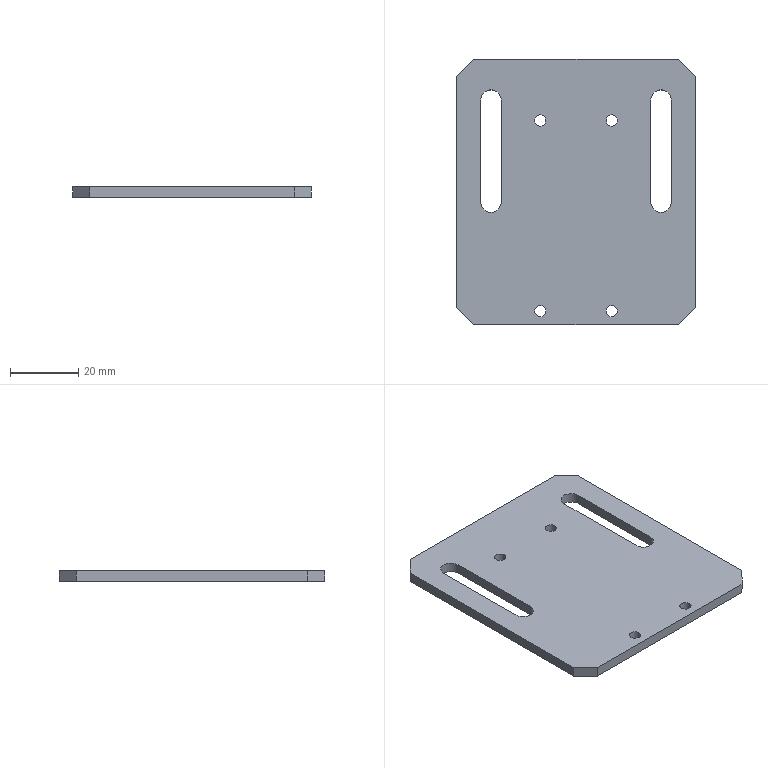Part | SolidWorks | features BaseBody 1 | 1 solid | 26 faces | box 70 x 78 x 3 mm | volume 14878 mm3 | plane 14 | cylinder 12 | commonest cylinder face diameters 3.3 x8 6 x4
STEP:
#1=CARTESIAN_POINT('',(8.85,-35.,-3.));
#2=VERTEX_POINT('',#1);
#3=CARTESIAN_POINT('',(12.15,-35.,-3.));
#4=VERTEX_POINT('',#3);
#5=CARTESIAN_POINT('',(10.5,-35.,-3.));
#6=DIRECTION('',(0.,0.,1.));
#7=DIRECTION('',(1.,0.,0.));
#8=AXIS2_PLACEMENT_3D('',#5,#6,#7);
#9=CIRCLE('',#8,1.65);
#10=EDGE_CURVE('',#2,#4,#9,.T.);
#11=ORIENTED_EDGE('',*,*,#10,.F.);
#12=CARTESIAN_POINT('',(8.85,-35.,0.));
#13=VERTEX_POINT('',#12);
#14=CARTESIAN_POINT('',(8.85,-35.,0.));
#15=DIRECTION('',(0.,0.,1.));
#16=VECTOR('',#15,1000.);
#17=LINE('',#14,#16);
#18=EDGE_CURVE('',#2,#13,#17,.T.);
#19=ORIENTED_EDGE('',*,*,#18,.T.);
#20=CARTESIAN_POINT('',(12.15,-35.,0.));
#21=VERTEX_POINT('',#20);
#22=CARTESIAN_POINT('',(10.5,-35.,0.));
#23=DIRECTION('',(0.,0.,-1.));
#24=DIRECTION('',(1.,0.,0.));
#25=AXIS2_PLACEMENT_3D('',#22,#23,#24);
#26=CIRCLE('',#25,1.65);
#27=EDGE_CURVE('',#21,#13,#26,.T.);
#28=ORIENTED_EDGE('',*,*,#27,.F.);
#29=CARTESIAN_POINT('',(12.15,-35.,0.));
#30=DIRECTION('',(0.,0.,1.));
#31=VECTOR('',#30,1000.);
#32=LINE('',#29,#31);
#33=EDGE_CURVE('',#4,#21,#32,.T.);
#34=ORIENTED_EDGE('',*,*,#33,.F.);
#35=EDGE_LOOP('',(#11,#19,#28,#34));
#36=FACE_OUTER_BOUND('',#35,.T.);
#37=CARTESIAN_POINT('',(10.5,-35.,0.));
#38=DIRECTION('',(0.,0.,1.));
#39=DIRECTION('',(1.,0.,0.));
#40=AXIS2_PLACEMENT_3D('',#37,#38,#39);
#41=CYLINDRICAL_SURFACE('',#40,1.65);
#42=ADVANCED_FACE('',(#36),#41,.F.);
#43=CARTESIAN_POINT('',(-12.15,-35.,-3.));
#44=VERTEX_POINT('',#43);
#45=CARTESIAN_POINT('',(-8.85,-35.,-3.));
#46=VERTEX_POINT('',#45);
#47=CARTESIAN_POINT('',(-10.5,-35.,-3.));
#48=DIRECTION('',(0.,0.,1.));
#49=DIRECTION('',(1.,0.,0.));
#50=AXIS2_PLACEMENT_3D('',#47,#48,#49);
#51=CIRCLE('',#50,1.65);
#52=EDGE_CURVE('',#44,#46,#51,.T.);
#53=ORIENTED_EDGE('',*,*,#52,.F.);
#54=CARTESIAN_POINT('',(-12.15,-35.,0.));
#55=VERTEX_POINT('',#54);
#56=CARTESIAN_POINT('',(-12.15,-35.,0.));
#57=DIRECTION('',(0.,0.,1.));
#58=VECTOR('',#57,1000.);
#59=LINE('',#56,#58);
#60=EDGE_CURVE('',#44,#55,#59,.T.);
#61=ORIENTED_EDGE('',*,*,#60,.T.);
#62=CARTESIAN_POINT('',(-8.85,-35.,0.));
#63=VERTEX_POINT('',#62);
#64=CARTESIAN_POINT('',(-10.5,-35.,0.));
#65=DIRECTION('',(0.,0.,-1.));
#66=DIRECTION('',(1.,0.,0.));
#67=AXIS2_PLACEMENT_3D('',#64,#65,#66);
#68=CIRCLE('',#67,1.65);
#69=EDGE_CURVE('',#63,#55,#68,.T.);
#70=ORIENTED_EDGE('',*,*,#69,.F.);
#71=CARTESIAN_POINT('',(-8.85,-35.,0.));
#72=DIRECTION('',(0.,0.,1.));
#73=VECTOR('',#72,1000.);
#74=LINE('',#71,#73);
#75=EDGE_CURVE('',#46,#63,#74,.T.);
#76=ORIENTED_EDGE('',*,*,#75,.F.);
#77=EDGE_LOOP('',(#53,#61,#70,#76));
#78=FACE_OUTER_BOUND('',#77,.T.);
#79=CARTESIAN_POINT('',(-10.5,-35.,0.));
#80=DIRECTION('',(0.,0.,1.));
#81=DIRECTION('',(1.,0.,0.));
#82=AXIS2_PLACEMENT_3D('',#79,#80,#81);
#83=CYLINDRICAL_SURFACE('',#82,1.65);
#84=ADVANCED_FACE('',(#78),#83,.F.);
#85=CARTESIAN_POINT('',(8.85,21.,-3.));
#86=VERTEX_POINT('',#85);
#87=CARTESIAN_POINT('',(12.15,21.,-3.));
#88=VERTEX_POINT('',#87);
#89=CARTESIAN_POINT('',(10.5,21.,-3.));
#90=DIRECTION('',(0.,0.,1.));
#91=DIRECTION('',(1.,0.,0.));
#92=AXIS2_PLACEMENT_3D('',#89,#90,#91);
#93=CIRCLE('',#92,1.65);
#94=EDGE_CURVE('',#86,#88,#93,.T.);
#95=ORIENTED_EDGE('',*,*,#94,.F.);
#96=CARTESIAN_POINT('',(8.85,21.,0.));
#97=VERTEX_POINT('',#96);
#98=CARTESIAN_POINT('',(8.85,21.,0.));
#99=DIRECTION('',(0.,0.,1.));
#100=VECTOR('',#99,1000.);
#101=LINE('',#98,#100);
#102=EDGE_CURVE('',#86,#97,#101,.T.);
#103=ORIENTED_EDGE('',*,*,#102,.T.);
#104=CARTESIAN_POINT('',(12.15,21.,0.));
#105=VERTEX_POINT('',#104);
#106=CARTESIAN_POINT('',(10.5,21.,0.));
#107=DIRECTION('',(0.,0.,-1.));
#108=DIRECTION('',(1.,0.,0.));
#109=AXIS2_PLACEMENT_3D('',#106,#107,#108);
#110=CIRCLE('',#109,1.65);
#111=EDGE_CURVE('',#105,#97,#110,.T.);
#112=ORIENTED_EDGE('',*,*,#111,.F.);
#113=CARTESIAN_POINT('',(12.15,21.,0.));
#114=DIRECTION('',(0.,0.,1.));
#115=VECTOR('',#114,1000.);
#116=LINE('',#113,#115);
#117=EDGE_CURVE('',#88,#105,#116,.T.);
#118=ORIENTED_EDGE('',*,*,#117,.F.);
#119=EDGE_LOOP('',(#95,#103,#112,#118));
#120=FACE_OUTER_BOUND('',#119,.T.);
#121=CARTESIAN_POINT('',(10.5,21.,0.));
#122=DIRECTION('',(0.,0.,1.));
#123=DIRECTION('',(1.,0.,0.));
#124=AXIS2_PLACEMENT_3D('',#121,#122,#123);
#125=CYLINDRICAL_SURFACE('',#124,1.65);
#126=ADVANCED_FACE('',(#120),#125,.F.);
#127=CARTESIAN_POINT('',(-12.15,21.,-3.));
#128=VERTEX_POINT('',#127);
#129=CARTESIAN_POINT('',(-8.85,21.,-3.));
#130=VERTEX_POINT('',#129);
#131=CARTESIAN_POINT('',(-10.5,21.,-3.));
#132=DIRECTION('',(0.,0.,1.));
#133=DIRECTION('',(1.,0.,0.));
#134=AXIS2_PLACEMENT_3D('',#131,#132,#133);
#135=CIRCLE('',#134,1.65);
#136=EDGE_CURVE('',#128,#130,#135,.T.);
#137=ORIENTED_EDGE('',*,*,#136,.F.);
#138=CARTESIAN_POINT('',(-12.15,21.,0.));
#139=VERTEX_POINT('',#138);
#140=CARTESIAN_POINT('',(-12.15,21.,0.));
#141=DIRECTION('',(0.,0.,1.));
#142=VECTOR('',#141,1000.);
#143=LINE('',#140,#142);
#144=EDGE_CURVE('',#128,#139,#143,.T.);
#145=ORIENTED_EDGE('',*,*,#144,.T.);
#146=CARTESIAN_POINT('',(-8.85,21.,0.));
#147=VERTEX_POINT('',#146);
#148=CARTESIAN_POINT('',(-10.5,21.,0.));
#149=DIRECTION('',(0.,0.,-1.));
#150=DIRECTION('',(1.,0.,0.));
#151=AXIS2_PLACEMENT_3D('',#148,#149,#150);
#152=CIRCLE('',#151,1.65);
#153=EDGE_CURVE('',#147,#139,#152,.T.);
#154=ORIENTED_EDGE('',*,*,#153,.F.);
#155=CARTESIAN_POINT('',(-8.85,21.,0.));
#156=DIRECTION('',(0.,0.,1.));
#157=VECTOR('',#156,1000.);
#158=LINE('',#155,#157);
#159=EDGE_CURVE('',#130,#147,#158,.T.);
#160=ORIENTED_EDGE('',*,*,#159,.F.);
#161=EDGE_LOOP('',(#137,#145,#154,#160));
#162=FACE_OUTER_BOUND('',#161,.T.);
#163=CARTESIAN_POINT('',(-10.5,21.,0.));
#164=DIRECTION('',(0.,0.,1.));
#165=DIRECTION('',(1.,0.,0.));
#166=AXIS2_PLACEMENT_3D('',#163,#164,#165);
#167=CYLINDRICAL_SURFACE('',#166,1.65);
#168=ADVANCED_FACE('',(#162),#167,.F.);
#169=CARTESIAN_POINT('',(30.,39.,0.));
#170=VERTEX_POINT('',#169);
#171=CARTESIAN_POINT('',(-30.,39.,0.));
#172=VERTEX_POINT('',#171);
#173=CARTESIAN_POINT('',(0.,39.,0.));
#174=DIRECTION('',(-1.,0.,0.));
#175=VECTOR('',#174,1000.);
#176=LINE('',#173,#175);
#177=EDGE_CURVE('',#170,#172,#176,.T.);
#178=ORIENTED_EDGE('',*,*,#177,.T.);
#179=CARTESIAN_POINT('',(-35.,34.,0.));
#180=VERTEX_POINT('',#179);
#181=CARTESIAN_POINT('',(-30.,39.,0.));
#182=DIRECTION('',(-0.7071,-0.7071,0.));
#183=VECTOR('',#182,1000.);
#184=LINE('',#181,#183);
#185=EDGE_CURVE('',#172,#180,#184,.T.);
#186=ORIENTED_EDGE('',*,*,#185,.T.);
#187=CARTESIAN_POINT('',(-35.,-34.,0.));
#188=VERTEX_POINT('',#187);
#189=CARTESIAN_POINT('',(-35.,0.,0.));
#190=DIRECTION('',(0.,-1.,0.));
#191=VECTOR('',#190,1000.);
#192=LINE('',#189,#191);
#193=EDGE_CURVE('',#180,#188,#192,.T.);
#194=ORIENTED_EDGE('',*,*,#193,.T.);
#195=CARTESIAN_POINT('',(-30.,-39.,0.));
#196=VERTEX_POINT('',#195);
#197=CARTESIAN_POINT('',(-35.,-34.,0.));
#198=DIRECTION('',(0.7071,-0.7071,0.));
#199=VECTOR('',#198,1000.);
#200=LINE('',#197,#199);
#201=EDGE_CURVE('',#188,#196,#200,.T.);
#202=ORIENTED_EDGE('',*,*,#201,.T.);
#203=CARTESIAN_POINT('',(30.,-39.,0.));
#204=VERTEX_POINT('',#203);
#205=CARTESIAN_POINT('',(0.,-39.,0.));
#206=DIRECTION('',(1.,0.,0.));
#207=VECTOR('',#206,1000.);
#208=LINE('',#205,#207);
#209=EDGE_CURVE('',#196,#204,#208,.T.);
#210=ORIENTED_EDGE('',*,*,#209,.T.);
#211=CARTESIAN_POINT('',(35.,-34.,0.));
#212=VERTEX_POINT('',#211);
#213=CARTESIAN_POINT('',(30.,-39.,0.));
#214=DIRECTION('',(0.7071,0.7071,0.));
#215=VECTOR('',#214,1000.);
#216=LINE('',#213,#215);
#217=EDGE_CURVE('',#204,#212,#216,.T.);
#218=ORIENTED_EDGE('',*,*,#217,.T.);
#219=CARTESIAN_POINT('',(35.,34.,0.));
#220=VERTEX_POINT('',#219);
#221=CARTESIAN_POINT('',(35.,0.,0.));
#222=DIRECTION('',(0.,1.,0.));
#223=VECTOR('',#222,1000.);
#224=LINE('',#221,#223);
#225=EDGE_CURVE('',#212,#220,#224,.T.);
#226=ORIENTED_EDGE('',*,*,#225,.T.);
#227=CARTESIAN_POINT('',(35.,34.,0.));
#228=DIRECTION('',(-0.7071,0.7071,0.));
#229=VECTOR('',#228,1000.);
#230=LINE('',#227,#229);
#231=EDGE_CURVE('',#220,#170,#230,.T.);
#232=ORIENTED_EDGE('',*,*,#231,.T.);
#233=EDGE_LOOP('',(#178,#186,#194,#202,#210,#218,#226,#232));
#234=FACE_OUTER_BOUND('',#233,.T.);
#235=ORIENTED_EDGE('',*,*,#27,.T.);
#236=CARTESIAN_POINT('',(10.5,-35.,0.));
#237=DIRECTION('',(0.,0.,-1.));
#238=DIRECTION('',(1.,0.,0.));
#239=AXIS2_PLACEMENT_3D('',#236,#237,#238);
#240=CIRCLE('',#239,1.65);
#241=EDGE_CURVE('',#13,#21,#240,.T.);
#242=ORIENTED_EDGE('',*,*,#241,.T.);
#243=EDGE_LOOP('',(#235,#242));
#244=FACE_BOUND('',#243,.T.);
#245=ORIENTED_EDGE('',*,*,#69,.T.);
#246=CARTESIAN_POINT('',(-10.5,-35.,0.));
#247=DIRECTION('',(0.,0.,-1.));
#248=DIRECTION('',(1.,0.,0.));
#249=AXIS2_PLACEMENT_3D('',#246,#247,#248);
#250=CIRCLE('',#249,1.65);
#251=EDGE_CURVE('',#55,#63,#250,.T.);
#252=ORIENTED_EDGE('',*,*,#251,.T.);
#253=EDGE_LOOP('',(#245,#252));
#254=FACE_BOUND('',#253,.T.);
#255=ORIENTED_EDGE('',*,*,#111,.T.);
#256=CARTESIAN_POINT('',(10.5,21.,0.));
#257=DIRECTION('',(0.,0.,-1.));
#258=DIRECTION('',(1.,0.,0.));
#259=AXIS2_PLACEMENT_3D('',#256,#257,#258);
#260=CIRCLE('',#259,1.65);
#261=EDGE_CURVE('',#97,#105,#260,.T.);
#262=ORIENTED_EDGE('',*,*,#261,.T.);
#263=EDGE_LOOP('',(#255,#262));
#264=FACE_BOUND('',#263,.T.);
#265=ORIENTED_EDGE('',*,*,#153,.T.);
#266=CARTESIAN_POINT('',(-10.5,21.,0.));
#267=DIRECTION('',(0.,0.,-1.));
#268=DIRECTION('',(1.,0.,0.));
#269=AXIS2_PLACEMENT_3D('',#266,#267,#268);
#270=CIRCLE('',#269,1.65);
#271=EDGE_CURVE('',#139,#147,#270,.T.);
#272=ORIENTED_EDGE('',*,*,#271,.T.);
#273=EDGE_LOOP('',(#265,#272));
#274=FACE_BOUND('',#273,.T.);
#275=CARTESIAN_POINT('',(-22.,-3.,0.));
#276=VERTEX_POINT('',#275);
#277=CARTESIAN_POINT('',(-28.,-3.,0.));
#278=VERTEX_POINT('',#277);
#279=CARTESIAN_POINT('',(-25.,-3.,0.));
#280=DIRECTION('',(0.,0.,-1.));
#281=DIRECTION('',(1.,0.,0.));
#282=AXIS2_PLACEMENT_3D('',#279,#280,#281);
#283=CIRCLE('',#282,3.);
#284=EDGE_CURVE('',#276,#278,#283,.T.);
#285=ORIENTED_EDGE('',*,*,#284,.T.);
#286=CARTESIAN_POINT('',(-28.,27.,0.));
#287=VERTEX_POINT('',#286);
#288=CARTESIAN_POINT('',(-28.,0.,0.));
#289=DIRECTION('',(0.,1.,0.));
#290=VECTOR('',#289,1000.);
#291=LINE('',#288,#290);
#292=EDGE_CURVE('',#278,#287,#291,.T.);
#293=ORIENTED_EDGE('',*,*,#292,.T.);
#294=CARTESIAN_POINT('',(-22.,27.,0.));
#295=VERTEX_POINT('',#294);
#296=CARTESIAN_POINT('',(-25.,27.,0.));
#297=DIRECTION('',(0.,0.,-1.));
#298=DIRECTION('',(1.,0.,0.));
#299=AXIS2_PLACEMENT_3D('',#296,#297,#298);
#300=CIRCLE('',#299,3.);
#301=EDGE_CURVE('',#287,#295,#300,.T.);
#302=ORIENTED_EDGE('',*,*,#301,.T.);
#303=CARTESIAN_POINT('',(-22.,0.,0.));
#304=DIRECTION('',(0.,-1.,0.));
#305=VECTOR('',#304,1000.);
#306=LINE('',#303,#305);
#307=EDGE_CURVE('',#295,#276,#306,.T.);
#308=ORIENTED_EDGE('',*,*,#307,.T.);
#309=EDGE_LOOP('',(#285,#293,#302,#308));
#310=FACE_BOUND('',#309,.T.);
#311=CARTESIAN_POINT('',(28.,-3.,0.));
#312=VERTEX_POINT('',#311);
#313=CARTESIAN_POINT('',(22.,-3.,0.));
#314=VERTEX_POINT('',#313);
#315=CARTESIAN_POINT('',(25.,-3.,0.));
#316=DIRECTION('',(0.,0.,-1.));
#317=DIRECTION('',(1.,0.,0.));
#318=AXIS2_PLACEMENT_3D('',#315,#316,#317);
#319=CIRCLE('',#318,3.);
#320=EDGE_CURVE('',#312,#314,#319,.T.);
#321=ORIENTED_EDGE('',*,*,#320,.T.);
#322=CARTESIAN_POINT('',(22.,27.,0.));
#323=VERTEX_POINT('',#322);
#324=CARTESIAN_POINT('',(22.,0.,0.));
#325=DIRECTION('',(0.,1.,0.));
#326=VECTOR('',#325,1000.);
#327=LINE('',#324,#326);
#328=EDGE_CURVE('',#314,#323,#327,.T.);
#329=ORIENTED_EDGE('',*,*,#328,.T.);
#330=CARTESIAN_POINT('',(28.,27.,0.));
#331=VERTEX_POINT('',#330);
#332=CARTESIAN_POINT('',(25.,27.,0.));
#333=DIRECTION('',(0.,0.,-1.));
#334=DIRECTION('',(1.,0.,0.));
#335=AXIS2_PLACEMENT_3D('',#332,#333,#334);
#336=CIRCLE('',#335,3.);
#337=EDGE_CURVE('',#323,#331,#336,.T.);
#338=ORIENTED_EDGE('',*,*,#337,.T.);
#339=CARTESIAN_POINT('',(28.,0.,0.));
#340=DIRECTION('',(0.,-1.,0.));
#341=VECTOR('',#340,1000.);
#342=LINE('',#339,#341);
#343=EDGE_CURVE('',#331,#312,#342,.T.);
#344=ORIENTED_EDGE('',*,*,#343,.T.);
#345=EDGE_LOOP('',(#321,#329,#338,#344));
#346=FACE_BOUND('',#345,.T.);
#347=CARTESIAN_POINT('',(0.,0.,0.));
#348=DIRECTION('',(0.,0.,1.));
#349=DIRECTION('',(1.,0.,0.));
#350=AXIS2_PLACEMENT_3D('',#347,#348,#349);
#351=PLANE('',#350);
#352=ADVANCED_FACE('',(#234,#244,#254,#264,#274,#310,#346),#351,.T.);
#353=CARTESIAN_POINT('',(-35.,34.,-3.));
#354=VERTEX_POINT('',#353);
#355=CARTESIAN_POINT('',(-35.,34.,-3.));
#356=DIRECTION('',(0.,0.,-1.));
#357=VECTOR('',#356,1000.);
#358=LINE('',#355,#357);
#359=EDGE_CURVE('',#180,#354,#358,.T.);
#360=ORIENTED_EDGE('',*,*,#359,.F.);
#361=ORIENTED_EDGE('',*,*,#185,.F.);
#362=CARTESIAN_POINT('',(-30.,39.,-3.));
#363=VERTEX_POINT('',#362);
#364=CARTESIAN_POINT('',(-30.,39.,-3.));
#365=DIRECTION('',(0.,0.,1.));
#366=VECTOR('',#365,1000.);
#367=LINE('',#364,#366);
#368=EDGE_CURVE('',#363,#172,#367,.T.);
#369=ORIENTED_EDGE('',*,*,#368,.F.);
#370=CARTESIAN_POINT('',(-30.,39.,-3.));
#371=DIRECTION('',(0.7071,0.7071,0.));
#372=VECTOR('',#371,1000.);
#373=LINE('',#370,#372);
#374=EDGE_CURVE('',#354,#363,#373,.T.);
#375=ORIENTED_EDGE('',*,*,#374,.F.);
#376=EDGE_LOOP('',(#360,#361,#369,#375));
#377=FACE_OUTER_BOUND('',#376,.T.);
#378=CARTESIAN_POINT('',(-30.,39.,-3.));
#379=DIRECTION('',(0.7071,-0.7071,0.));
#380=DIRECTION('',(0.7071,0.7071,0.));
#381=AXIS2_PLACEMENT_3D('',#378,#379,#380);
#382=PLANE('',#381);
#383=ADVANCED_FACE('',(#377),#382,.F.);
#384=CARTESIAN_POINT('',(30.,39.,-3.));
#385=VERTEX_POINT('',#384);
#386=CARTESIAN_POINT('',(-35.,39.,-3.));
#387=DIRECTION('',(-1.,0.,0.));
#388=VECTOR('',#387,1000.);
#389=LINE('',#386,#388);
#390=EDGE_CURVE('',#385,#363,#389,.T.);
#391=ORIENTED_EDGE('',*,*,#390,.T.);
#392=ORIENTED_EDGE('',*,*,#368,.T.);
#393=ORIENTED_EDGE('',*,*,#177,.F.);
#394=CARTESIAN_POINT('',(30.,39.,-3.));
#395=DIRECTION('',(0.,0.,-1.));
#396=VECTOR('',#395,1000.);
#397=LINE('',#394,#396);
#398=EDGE_CURVE('',#170,#385,#397,.T.);
#399=ORIENTED_EDGE('',*,*,#398,.T.);
#400=EDGE_LOOP('',(#391,#392,#393,#399));
#401=FACE_OUTER_BOUND('',#400,.T.);
#402=CARTESIAN_POINT('',(-35.,39.,-3.));
#403=DIRECTION('',(0.,1.,0.));
#404=DIRECTION('',(0.,0.,1.));
#405=AXIS2_PLACEMENT_3D('',#402,#403,#404);
#406=PLANE('',#405);
#407=ADVANCED_FACE('',(#401),#406,.T.);
#408=ORIENTED_EDGE('',*,*,#398,.F.);
#409=ORIENTED_EDGE('',*,*,#231,.F.);
#410=CARTESIAN_POINT('',(35.,34.,-3.));
#411=VERTEX_POINT('',#410);
#412=CARTESIAN_POINT('',(35.,34.,-3.));
#413=DIRECTION('',(0.,0.,1.));
#414=VECTOR('',#413,1000.);
#415=LINE('',#412,#414);
#416=EDGE_CURVE('',#411,#220,#415,.T.);
#417=ORIENTED_EDGE('',*,*,#416,.F.);
#418=CARTESIAN_POINT('',(35.,34.,-3.));
#419=DIRECTION('',(0.7071,-0.7071,0.));
#420=VECTOR('',#419,1000.);
#421=LINE('',#418,#420);
#422=EDGE_CURVE('',#385,#411,#421,.T.);
#423=ORIENTED_EDGE('',*,*,#422,.F.);
#424=EDGE_LOOP('',(#408,#409,#417,#423));
#425=FACE_OUTER_BOUND('',#424,.T.);
#426=CARTESIAN_POINT('',(35.,34.,-3.));
#427=DIRECTION('',(-0.7071,-0.7071,0.));
#428=DIRECTION('',(0.7071,-0.7071,0.));
#429=AXIS2_PLACEMENT_3D('',#426,#427,#428);
#430=PLANE('',#429);
#431=ADVANCED_FACE('',(#425),#430,.F.);
#432=CARTESIAN_POINT('',(35.,-34.,-3.));
#433=VERTEX_POINT('',#432);
#434=CARTESIAN_POINT('',(35.,39.,-3.));
#435=DIRECTION('',(0.,1.,0.));
#436=VECTOR('',#435,1000.);
#437=LINE('',#434,#436);
#438=EDGE_CURVE('',#433,#411,#437,.T.);
#439=ORIENTED_EDGE('',*,*,#438,.T.);
#440=ORIENTED_EDGE('',*,*,#416,.T.);
#441=ORIENTED_EDGE('',*,*,#225,.F.);
#442=CARTESIAN_POINT('',(35.,-34.,-3.));
#443=DIRECTION('',(0.,0.,-1.));
#444=VECTOR('',#443,1000.);
#445=LINE('',#442,#444);
#446=EDGE_CURVE('',#212,#433,#445,.T.);
#447=ORIENTED_EDGE('',*,*,#446,.T.);
#448=EDGE_LOOP('',(#439,#440,#441,#447));
#449=FACE_OUTER_BOUND('',#448,.T.);
#450=CARTESIAN_POINT('',(35.,39.,-3.));
#451=DIRECTION('',(1.,0.,0.));
#452=DIRECTION('',(0.,1.,0.));
#453=AXIS2_PLACEMENT_3D('',#450,#451,#452);
#454=PLANE('',#453);
#455=ADVANCED_FACE('',(#449),#454,.T.);
#456=ORIENTED_EDGE('',*,*,#446,.F.);
#457=ORIENTED_EDGE('',*,*,#217,.F.);
#458=CARTESIAN_POINT('',(30.,-39.,-3.));
#459=VERTEX_POINT('',#458);
#460=CARTESIAN_POINT('',(30.,-39.,-3.));
#461=DIRECTION('',(0.,0.,1.));
#462=VECTOR('',#461,1000.);
#463=LINE('',#460,#462);
#464=EDGE_CURVE('',#459,#204,#463,.T.);
#465=ORIENTED_EDGE('',*,*,#464,.F.);
#466=CARTESIAN_POINT('',(30.,-39.,-3.));
#467=DIRECTION('',(-0.7071,-0.7071,0.));
#468=VECTOR('',#467,1000.);
#469=LINE('',#466,#468);
#470=EDGE_CURVE('',#433,#459,#469,.T.);
#471=ORIENTED_EDGE('',*,*,#470,.F.);
#472=EDGE_LOOP('',(#456,#457,#465,#471));
#473=FACE_OUTER_BOUND('',#472,.T.);
#474=CARTESIAN_POINT('',(30.,-39.,-3.));
#475=DIRECTION('',(-0.7071,0.7071,0.));
#476=DIRECTION('',(-0.7071,-0.7071,0.));
#477=AXIS2_PLACEMENT_3D('',#474,#475,#476);
#478=PLANE('',#477);
#479=ADVANCED_FACE('',(#473),#478,.F.);
#480=CARTESIAN_POINT('',(-30.,-39.,-3.));
#481=VERTEX_POINT('',#480);
#482=CARTESIAN_POINT('',(-35.,-39.,-3.));
#483=DIRECTION('',(1.,0.,0.));
#484=VECTOR('',#483,1000.);
#485=LINE('',#482,#484);
#486=EDGE_CURVE('',#481,#459,#485,.T.);
#487=ORIENTED_EDGE('',*,*,#486,.T.);
#488=ORIENTED_EDGE('',*,*,#464,.T.);
#489=ORIENTED_EDGE('',*,*,#209,.F.);
#490=CARTESIAN_POINT('',(-30.,-39.,-3.));
#491=DIRECTION('',(0.,0.,-1.));
#492=VECTOR('',#491,1000.);
#493=LINE('',#490,#492);
#494=EDGE_CURVE('',#196,#481,#493,.T.);
#495=ORIENTED_EDGE('',*,*,#494,.T.);
#496=EDGE_LOOP('',(#487,#488,#489,#495));
#497=FACE_OUTER_BOUND('',#496,.T.);
#498=CARTESIAN_POINT('',(-35.,-39.,-3.));
#499=DIRECTION('',(0.,-1.,0.));
#500=DIRECTION('',(0.,0.,-1.));
#501=AXIS2_PLACEMENT_3D('',#498,#499,#500);
#502=PLANE('',#501);
#503=ADVANCED_FACE('',(#497),#502,.T.);
#504=ORIENTED_EDGE('',*,*,#494,.F.);
#505=ORIENTED_EDGE('',*,*,#201,.F.);
#506=CARTESIAN_POINT('',(-35.,-34.,-3.));
#507=VERTEX_POINT('',#506);
#508=CARTESIAN_POINT('',(-35.,-34.,-3.));
#509=DIRECTION('',(0.,0.,1.));
#510=VECTOR('',#509,1000.);
#511=LINE('',#508,#510);
#512=EDGE_CURVE('',#507,#188,#511,.T.);
#513=ORIENTED_EDGE('',*,*,#512,.F.);
#514=CARTESIAN_POINT('',(-35.,-34.,-3.));
#515=DIRECTION('',(-0.7071,0.7071,0.));
#516=VECTOR('',#515,1000.);
#517=LINE('',#514,#516);
#518=EDGE_CURVE('',#481,#507,#517,.T.);
#519=ORIENTED_EDGE('',*,*,#518,.F.);
#520=EDGE_LOOP('',(#504,#505,#513,#519));
#521=FACE_OUTER_BOUND('',#520,.T.);
#522=CARTESIAN_POINT('',(-35.,-34.,-3.));
#523=DIRECTION('',(0.7071,0.7071,0.));
#524=DIRECTION('',(-0.7071,0.7071,0.));
#525=AXIS2_PLACEMENT_3D('',#522,#523,#524);
#526=PLANE('',#525);
#527=ADVANCED_FACE('',(#521),#526,.F.);
#528=ORIENTED_EDGE('',*,*,#193,.F.);
#529=ORIENTED_EDGE('',*,*,#359,.T.);
#530=CARTESIAN_POINT('',(-35.,39.,-3.));
#531=DIRECTION('',(0.,-1.,0.));
#532=VECTOR('',#531,1000.);
#533=LINE('',#530,#532);
#534=EDGE_CURVE('',#354,#507,#533,.T.);
#535=ORIENTED_EDGE('',*,*,#534,.T.);
#536=ORIENTED_EDGE('',*,*,#512,.T.);
#537=EDGE_LOOP('',(#528,#529,#535,#536));
#538=FACE_OUTER_BOUND('',#537,.T.);
#539=CARTESIAN_POINT('',(-35.,39.,-3.));
#540=DIRECTION('',(-1.,0.,0.));
#541=DIRECTION('',(0.,-1.,0.));
#542=AXIS2_PLACEMENT_3D('',#539,#540,#541);
#543=PLANE('',#542);
#544=ADVANCED_FACE('',(#538),#543,.T.);
#545=ORIENTED_EDGE('',*,*,#18,.F.);
#546=CARTESIAN_POINT('',(10.5,-35.,-3.));
#547=DIRECTION('',(0.,0.,1.));
#548=DIRECTION('',(1.,0.,0.));
#549=AXIS2_PLACEMENT_3D('',#546,#547,#548);
#550=CIRCLE('',#549,1.65);
#551=EDGE_CURVE('',#4,#2,#550,.T.);
#552=ORIENTED_EDGE('',*,*,#551,.F.);
#553=ORIENTED_EDGE('',*,*,#33,.T.);
#554=ORIENTED_EDGE('',*,*,#241,.F.);
#555=EDGE_LOOP('',(#545,#552,#553,#554));
#556=FACE_OUTER_BOUND('',#555,.T.);
#557=CARTESIAN_POINT('',(10.5,-35.,0.));
#558=DIRECTION('',(0.,0.,1.));
#559=DIRECTION('',(1.,0.,0.));
#560=AXIS2_PLACEMENT_3D('',#557,#558,#559);
#561=CYLINDRICAL_SURFACE('',#560,1.65);
#562=ADVANCED_FACE('',(#556),#561,.F.);
#563=ORIENTED_EDGE('',*,*,#60,.F.);
#564=CARTESIAN_POINT('',(-10.5,-35.,-3.));
#565=DIRECTION('',(0.,0.,1.));
#566=DIRECTION('',(1.,0.,0.));
#567=AXIS2_PLACEMENT_3D('',#564,#565,#566);
#568=CIRCLE('',#567,1.65);
#569=EDGE_CURVE('',#46,#44,#568,.T.);
#570=ORIENTED_EDGE('',*,*,#569,.F.);
#571=ORIENTED_EDGE('',*,*,#75,.T.);
#572=ORIENTED_EDGE('',*,*,#251,.F.);
#573=EDGE_LOOP('',(#563,#570,#571,#572));
#574=FACE_OUTER_BOUND('',#573,.T.);
#575=CARTESIAN_POINT('',(-10.5,-35.,0.));
#576=DIRECTION('',(0.,0.,1.));
#577=DIRECTION('',(1.,0.,0.));
#578=AXIS2_PLACEMENT_3D('',#575,#576,#577);
#579=CYLINDRICAL_SURFACE('',#578,1.65);
#580=ADVANCED_FACE('',(#574),#579,.F.);
#581=ORIENTED_EDGE('',*,*,#102,.F.);
#582=CARTESIAN_POINT('',(10.5,21.,-3.));
#583=DIRECTION('',(0.,0.,1.));
#584=DIRECTION('',(1.,0.,0.));
#585=AXIS2_PLACEMENT_3D('',#582,#583,#584);
#586=CIRCLE('',#585,1.65);
#587=EDGE_CURVE('',#88,#86,#586,.T.);
#588=ORIENTED_EDGE('',*,*,#587,.F.);
#589=ORIENTED_EDGE('',*,*,#117,.T.);
#590=ORIENTED_EDGE('',*,*,#261,.F.);
#591=EDGE_LOOP('',(#581,#588,#589,#590));
#592=FACE_OUTER_BOUND('',#591,.T.);
#593=CARTESIAN_POINT('',(10.5,21.,0.));
#594=DIRECTION('',(0.,0.,1.));
#595=DIRECTION('',(1.,0.,0.));
#596=AXIS2_PLACEMENT_3D('',#593,#594,#595);
#597=CYLINDRICAL_SURFACE('',#596,1.65);
#598=ADVANCED_FACE('',(#592),#597,.F.);
#599=ORIENTED_EDGE('',*,*,#144,.F.);
#600=CARTESIAN_POINT('',(-10.5,21.,-3.));
#601=DIRECTION('',(0.,0.,1.));
#602=DIRECTION('',(1.,0.,0.));
#603=AXIS2_PLACEMENT_3D('',#600,#601,#602);
#604=CIRCLE('',#603,1.65);
#605=EDGE_CURVE('',#130,#128,#604,.T.);
#606=ORIENTED_EDGE('',*,*,#605,.F.);
#607=ORIENTED_EDGE('',*,*,#159,.T.);
#608=ORIENTED_EDGE('',*,*,#271,.F.);
#609=EDGE_LOOP('',(#599,#606,#607,#608));
#610=FACE_OUTER_BOUND('',#609,.T.);
#611=CARTESIAN_POINT('',(-10.5,21.,0.));
#612=DIRECTION('',(0.,0.,1.));
#613=DIRECTION('',(1.,0.,0.));
#614=AXIS2_PLACEMENT_3D('',#611,#612,#613);
#615=CYLINDRICAL_SURFACE('',#614,1.65);
#616=ADVANCED_FACE('',(#610),#615,.F.);
#617=CARTESIAN_POINT('',(-28.,-3.,-3.));
#618=VERTEX_POINT('',#617);
#619=CARTESIAN_POINT('',(-28.,-3.,-3.));
#620=DIRECTION('',(0.,0.,1.));
#621=VECTOR('',#620,1000.);
#622=LINE('',#619,#621);
#623=EDGE_CURVE('',#618,#278,#622,.T.);
#624=ORIENTED_EDGE('',*,*,#623,.F.);
#625=CARTESIAN_POINT('',(-28.,27.,-3.));
#626=VERTEX_POINT('',#625);
#627=CARTESIAN_POINT('',(-28.,27.,-3.));
#628=DIRECTION('',(0.,-1.,0.));
#629=VECTOR('',#628,1000.);
#630=LINE('',#627,#629);
#631=EDGE_CURVE('',#626,#618,#630,.T.);
#632=ORIENTED_EDGE('',*,*,#631,.F.);
#633=CARTESIAN_POINT('',(-28.,27.,-3.));
#634=DIRECTION('',(0.,0.,-1.));
#635=VECTOR('',#634,1000.);
#636=LINE('',#633,#635);
#637=EDGE_CURVE('',#287,#626,#636,.T.);
#638=ORIENTED_EDGE('',*,*,#637,.F.);
#639=ORIENTED_EDGE('',*,*,#292,.F.);
#640=EDGE_LOOP('',(#624,#632,#638,#639));
#641=FACE_OUTER_BOUND('',#640,.T.);
#642=CARTESIAN_POINT('',(-28.,27.,-3.));
#643=DIRECTION('',(-1.,0.,0.));
#644=DIRECTION('',(0.,-1.,0.));
#645=AXIS2_PLACEMENT_3D('',#642,#643,#644);
#646=PLANE('',#645);
#647=ADVANCED_FACE('',(#641),#646,.F.);
#648=CARTESIAN_POINT('',(-22.,-3.,-3.));
#649=VERTEX_POINT('',#648);
#650=CARTESIAN_POINT('',(-22.,-3.,-3.));
#651=DIRECTION('',(0.,0.,1.));
#652=VECTOR('',#651,1000.);
#653=LINE('',#650,#652);
#654=EDGE_CURVE('',#649,#276,#653,.T.);
#655=ORIENTED_EDGE('',*,*,#654,.F.);
#656=CARTESIAN_POINT('',(-25.,-3.,-3.));
#657=DIRECTION('',(0.,0.,1.));
#658=DIRECTION('',(1.,0.,0.));
#659=AXIS2_PLACEMENT_3D('',#656,#657,#658);
#660=CIRCLE('',#659,3.);
#661=EDGE_CURVE('',#618,#649,#660,.T.);
#662=ORIENTED_EDGE('',*,*,#661,.F.);
#663=ORIENTED_EDGE('',*,*,#623,.T.);
#664=ORIENTED_EDGE('',*,*,#284,.F.);
#665=EDGE_LOOP('',(#655,#662,#663,#664));
#666=FACE_OUTER_BOUND('',#665,.T.);
#667=CARTESIAN_POINT('',(-25.,-3.,-3.));
#668=DIRECTION('',(0.,0.,1.));
#669=DIRECTION('',(1.,0.,0.));
#670=AXIS2_PLACEMENT_3D('',#667,#668,#669);
#671=CYLINDRICAL_SURFACE('',#670,3.);
#672=ADVANCED_FACE('',(#666),#671,.F.);
#673=CARTESIAN_POINT('',(-22.,27.,-3.));
#674=VERTEX_POINT('',#673);
#675=CARTESIAN_POINT('',(-22.,27.,-3.));
#676=DIRECTION('',(0.,0.,1.));
#677=VECTOR('',#676,1000.);
#678=LINE('',#675,#677);
#679=EDGE_CURVE('',#674,#295,#678,.T.);
#680=ORIENTED_EDGE('',*,*,#679,.F.);
#681=CARTESIAN_POINT('',(-22.,27.,-3.));
#682=DIRECTION('',(0.,1.,0.));
#683=VECTOR('',#682,1000.);
#684=LINE('',#681,#683);
#685=EDGE_CURVE('',#649,#674,#684,.T.);
#686=ORIENTED_EDGE('',*,*,#685,.F.);
#687=ORIENTED_EDGE('',*,*,#654,.T.);
#688=ORIENTED_EDGE('',*,*,#307,.F.);
#689=EDGE_LOOP('',(#680,#686,#687,#688));
#690=FACE_OUTER_BOUND('',#689,.T.);
#691=CARTESIAN_POINT('',(-22.,27.,-3.));
#692=DIRECTION('',(1.,0.,0.));
#693=DIRECTION('',(0.,1.,0.));
#694=AXIS2_PLACEMENT_3D('',#691,#692,#693);
#695=PLANE('',#694);
#696=ADVANCED_FACE('',(#690),#695,.F.);
#697=ORIENTED_EDGE('',*,*,#637,.T.);
#698=CARTESIAN_POINT('',(-25.,27.,-3.));
#699=DIRECTION('',(0.,0.,1.));
#700=DIRECTION('',(1.,0.,0.));
#701=AXIS2_PLACEMENT_3D('',#698,#699,#700);
#702=CIRCLE('',#701,3.);
#703=EDGE_CURVE('',#674,#626,#702,.T.);
#704=ORIENTED_EDGE('',*,*,#703,.F.);
#705=ORIENTED_EDGE('',*,*,#679,.T.);
#706=ORIENTED_EDGE('',*,*,#301,.F.);
#707=EDGE_LOOP('',(#697,#704,#705,#706));
#708=FACE_OUTER_BOUND('',#707,.T.);
#709=CARTESIAN_POINT('',(-25.,27.,-3.));
#710=DIRECTION('',(0.,0.,1.));
#711=DIRECTION('',(1.,0.,0.));
#712=AXIS2_PLACEMENT_3D('',#709,#710,#711);
#713=CYLINDRICAL_SURFACE('',#712,3.);
#714=ADVANCED_FACE('',(#708),#713,.F.);
#715=CARTESIAN_POINT('',(22.,-3.,-3.));
#716=VERTEX_POINT('',#715);
#717=CARTESIAN_POINT('',(22.,-3.,-3.));
#718=DIRECTION('',(0.,0.,1.));
#719=VECTOR('',#718,1000.);
#720=LINE('',#717,#719);
#721=EDGE_CURVE('',#716,#314,#720,.T.);
#722=ORIENTED_EDGE('',*,*,#721,.F.);
#723=CARTESIAN_POINT('',(22.,27.,-3.));
#724=VERTEX_POINT('',#723);
#725=CARTESIAN_POINT('',(22.,27.,-3.));
#726=DIRECTION('',(0.,-1.,0.));
#727=VECTOR('',#726,1000.);
#728=LINE('',#725,#727);
#729=EDGE_CURVE('',#724,#716,#728,.T.);
#730=ORIENTED_EDGE('',*,*,#729,.F.);
#731=CARTESIAN_POINT('',(22.,27.,-3.));
#732=DIRECTION('',(0.,0.,-1.));
#733=VECTOR('',#732,1000.);
#734=LINE('',#731,#733);
#735=EDGE_CURVE('',#323,#724,#734,.T.);
#736=ORIENTED_EDGE('',*,*,#735,.F.);
#737=ORIENTED_EDGE('',*,*,#328,.F.);
#738=EDGE_LOOP('',(#722,#730,#736,#737));
#739=FACE_OUTER_BOUND('',#738,.T.);
#740=CARTESIAN_POINT('',(22.,27.,-3.));
#741=DIRECTION('',(-1.,0.,0.));
#742=DIRECTION('',(0.,-1.,0.));
#743=AXIS2_PLACEMENT_3D('',#740,#741,#742);
#744=PLANE('',#743);
#745=ADVANCED_FACE('',(#739),#744,.F.);
#746=CARTESIAN_POINT('',(28.,-3.,-3.));
#747=VERTEX_POINT('',#746);
#748=CARTESIAN_POINT('',(28.,-3.,-3.));
#749=DIRECTION('',(0.,0.,1.));
#750=VECTOR('',#749,1000.);
#751=LINE('',#748,#750);
#752=EDGE_CURVE('',#747,#312,#751,.T.);
#753=ORIENTED_EDGE('',*,*,#752,.F.);
#754=CARTESIAN_POINT('',(25.,-3.,-3.));
#755=DIRECTION('',(0.,0.,1.));
#756=DIRECTION('',(1.,0.,0.));
#757=AXIS2_PLACEMENT_3D('',#754,#755,#756);
#758=CIRCLE('',#757,3.);
#759=EDGE_CURVE('',#716,#747,#758,.T.);
#760=ORIENTED_EDGE('',*,*,#759,.F.);
#761=ORIENTED_EDGE('',*,*,#721,.T.);
#762=ORIENTED_EDGE('',*,*,#320,.F.);
#763=EDGE_LOOP('',(#753,#760,#761,#762));
#764=FACE_OUTER_BOUND('',#763,.T.);
#765=CARTESIAN_POINT('',(25.,-3.,-3.));
#766=DIRECTION('',(0.,0.,1.));
#767=DIRECTION('',(1.,0.,0.));
#768=AXIS2_PLACEMENT_3D('',#765,#766,#767);
#769=CYLINDRICAL_SURFACE('',#768,3.);
#770=ADVANCED_FACE('',(#764),#769,.F.);
#771=CARTESIAN_POINT('',(28.,27.,-3.));
#772=VERTEX_POINT('',#771);
#773=CARTESIAN_POINT('',(28.,27.,-3.));
#774=DIRECTION('',(0.,0.,1.));
#775=VECTOR('',#774,1000.);
#776=LINE('',#773,#775);
#777=EDGE_CURVE('',#772,#331,#776,.T.);
#778=ORIENTED_EDGE('',*,*,#777,.F.);
#779=CARTESIAN_POINT('',(28.,27.,-3.));
#780=DIRECTION('',(0.,1.,0.));
#781=VECTOR('',#780,1000.);
#782=LINE('',#779,#781);
#783=EDGE_CURVE('',#747,#772,#782,.T.);
#784=ORIENTED_EDGE('',*,*,#783,.F.);
#785=ORIENTED_EDGE('',*,*,#752,.T.);
#786=ORIENTED_EDGE('',*,*,#343,.F.);
#787=EDGE_LOOP('',(#778,#784,#785,#786));
#788=FACE_OUTER_BOUND('',#787,.T.);
#789=CARTESIAN_POINT('',(28.,27.,-3.));
#790=DIRECTION('',(1.,0.,0.));
#791=DIRECTION('',(0.,1.,0.));
#792=AXIS2_PLACEMENT_3D('',#789,#790,#791);
#793=PLANE('',#792);
#794=ADVANCED_FACE('',(#788),#793,.F.);
#795=ORIENTED_EDGE('',*,*,#735,.T.);
#796=CARTESIAN_POINT('',(25.,27.,-3.));
#797=DIRECTION('',(0.,0.,1.));
#798=DIRECTION('',(1.,0.,0.));
#799=AXIS2_PLACEMENT_3D('',#796,#797,#798);
#800=CIRCLE('',#799,3.);
#801=EDGE_CURVE('',#772,#724,#800,.T.);
#802=ORIENTED_EDGE('',*,*,#801,.F.);
#803=ORIENTED_EDGE('',*,*,#777,.T.);
#804=ORIENTED_EDGE('',*,*,#337,.F.);
#805=EDGE_LOOP('',(#795,#802,#803,#804));
#806=FACE_OUTER_BOUND('',#805,.T.);
#807=CARTESIAN_POINT('',(25.,27.,-3.));
#808=DIRECTION('',(0.,0.,1.));
#809=DIRECTION('',(1.,0.,0.));
#810=AXIS2_PLACEMENT_3D('',#807,#808,#809);
#811=CYLINDRICAL_SURFACE('',#810,3.);
#812=ADVANCED_FACE('',(#806),#811,.F.);
#813=ORIENTED_EDGE('',*,*,#518,.T.);
#814=ORIENTED_EDGE('',*,*,#534,.F.);
#815=ORIENTED_EDGE('',*,*,#374,.T.);
#816=ORIENTED_EDGE('',*,*,#390,.F.);
#817=ORIENTED_EDGE('',*,*,#422,.T.);
#818=ORIENTED_EDGE('',*,*,#438,.F.);
#819=ORIENTED_EDGE('',*,*,#470,.T.);
#820=ORIENTED_EDGE('',*,*,#486,.F.);
#821=EDGE_LOOP('',(#813,#814,#815,#816,#817,#818,#819,#820));
#822=FACE_OUTER_BOUND('',#821,.T.);
#823=ORIENTED_EDGE('',*,*,#551,.T.);
#824=ORIENTED_EDGE('',*,*,#10,.T.);
#825=EDGE_LOOP('',(#823,#824));
#826=FACE_BOUND('',#825,.T.);
#827=ORIENTED_EDGE('',*,*,#569,.T.);
#828=ORIENTED_EDGE('',*,*,#52,.T.);
#829=EDGE_LOOP('',(#827,#828));
#830=FACE_BOUND('',#829,.T.);
#831=ORIENTED_EDGE('',*,*,#587,.T.);
#832=ORIENTED_EDGE('',*,*,#94,.T.);
#833=EDGE_LOOP('',(#831,#832));
#834=FACE_BOUND('',#833,.T.);
#835=ORIENTED_EDGE('',*,*,#605,.T.);
#836=ORIENTED_EDGE('',*,*,#136,.T.);
#837=EDGE_LOOP('',(#835,#836));
#838=FACE_BOUND('',#837,.T.);
#839=ORIENTED_EDGE('',*,*,#703,.T.);
#840=ORIENTED_EDGE('',*,*,#631,.T.);
#841=ORIENTED_EDGE('',*,*,#661,.T.);
#842=ORIENTED_EDGE('',*,*,#685,.T.);
#843=EDGE_LOOP('',(#839,#840,#841,#842));
#844=FACE_BOUND('',#843,.T.);
#845=ORIENTED_EDGE('',*,*,#801,.T.);
#846=ORIENTED_EDGE('',*,*,#729,.T.);
#847=ORIENTED_EDGE('',*,*,#759,.T.);
#848=ORIENTED_EDGE('',*,*,#783,.T.);
#849=EDGE_LOOP('',(#845,#846,#847,#848));
#850=FACE_BOUND('',#849,.T.);
#851=CARTESIAN_POINT('',(0.,0.,-3.));
#852=DIRECTION('',(0.,0.,1.));
#853=DIRECTION('',(1.,0.,0.));
#854=AXIS2_PLACEMENT_3D('',#851,#852,#853);
#855=PLANE('',#854);
#856=ADVANCED_FACE('',(#822,#826,#830,#834,#838,#844,#850),#855,.F.);
#857=CLOSED_SHELL('',(#42,#84,#126,#168,#352,#383,#407,#431,#455,#479,#503,#527,#544,#562,#580,#598,#616,#647,#672,#696,#714,#745,#770,#794,#812,#856));
#858=MANIFOLD_SOLID_BREP('',#857);
#859=CARTESIAN_POINT('',(0.,0.,0.));
#860=DIRECTION('',(0.,0.,1.));
#861=DIRECTION('',(1.,0.,0.));
#862=AXIS2_PLACEMENT_3D('',#859,#860,#861);
#863=(LENGTH_UNIT()NAMED_UNIT(*)SI_UNIT(.MILLI.,.METRE.));
#864=UNCERTAINTY_MEASURE_WITH_UNIT(LENGTH_MEASURE(0.00001),#863,'','');
#865=(NAMED_UNIT(*)PLANE_ANGLE_UNIT()SI_UNIT($,.RADIAN.));
#866=(NAMED_UNIT(*)SI_UNIT($,.STERADIAN.)SOLID_ANGLE_UNIT());
#867=(GEOMETRIC_REPRESENTATION_CONTEXT(3)GLOBAL_UNCERTAINTY_ASSIGNED_CONTEXT((#864))GLOBAL_UNIT_ASSIGNED_CONTEXT((#863,#865,#866))REPRESENTATION_CONTEXT('',''));
#868=ADVANCED_BREP_SHAPE_REPRESENTATION('',(#858,#862),#867);